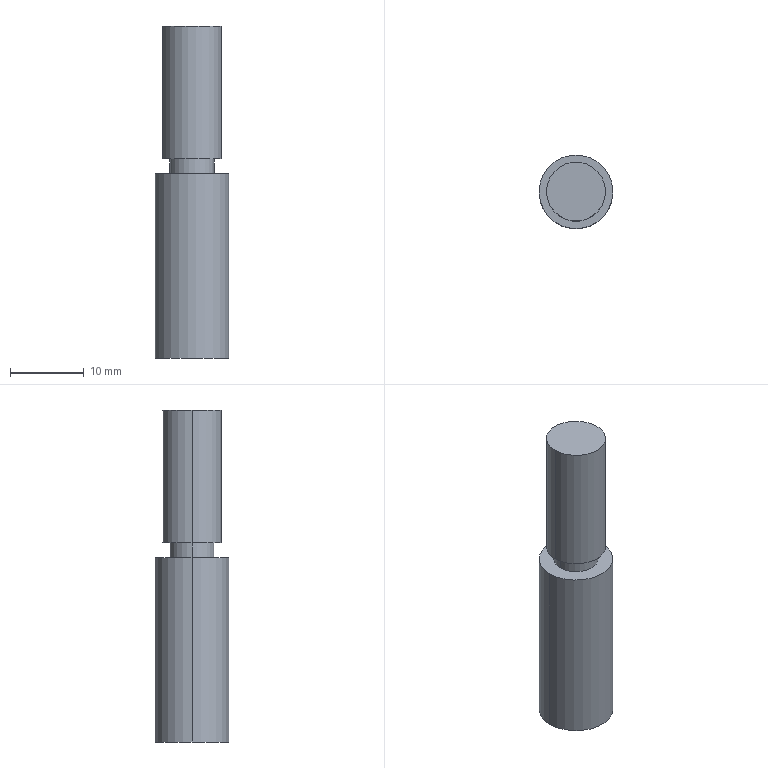Part | SolidWorks | features ICE 2, Extrusion 1 | 1 solid | 10 faces | box 10 x 10 x 45 mm | volume 2925 mm3 | cylinder 6 | plane 4 | commonest cylinder face diameters 6 x2 8 x2 10 x2
STEP:
#1=CARTESIAN_POINT('',(4.,0.,45.));
#2=VERTEX_POINT('',#1);
#3=CARTESIAN_POINT('',(-4.,0.,45.));
#4=VERTEX_POINT('',#3);
#5=CARTESIAN_POINT('',(0.,0.,45.));
#6=DIRECTION('',(0.,0.,1.));
#7=DIRECTION('',(1.,0.,0.));
#8=AXIS2_PLACEMENT_3D('',#5,#6,#7);
#9=CIRCLE('',#8,4.);
#10=EDGE_CURVE('',#2,#4,#9,.T.);
#11=ORIENTED_EDGE('',*,*,#10,.F.);
#12=CARTESIAN_POINT('',(4.,0.,27.));
#13=VERTEX_POINT('',#12);
#14=CARTESIAN_POINT('',(4.,0.,45.));
#15=DIRECTION('',(0.,0.,-1.));
#16=VECTOR('',#15,1000.);
#17=LINE('',#14,#16);
#18=EDGE_CURVE('',#2,#13,#17,.T.);
#19=ORIENTED_EDGE('',*,*,#18,.T.);
#20=CARTESIAN_POINT('',(-4.,0.,27.));
#21=VERTEX_POINT('',#20);
#22=CARTESIAN_POINT('',(0.,0.,27.));
#23=DIRECTION('',(0.,0.,1.));
#24=DIRECTION('',(1.,0.,0.));
#25=AXIS2_PLACEMENT_3D('',#22,#23,#24);
#26=CIRCLE('',#25,4.);
#27=EDGE_CURVE('',#13,#21,#26,.T.);
#28=ORIENTED_EDGE('',*,*,#27,.T.);
#29=CARTESIAN_POINT('',(-4.,0.,45.));
#30=DIRECTION('',(0.,0.,-1.));
#31=VECTOR('',#30,1000.);
#32=LINE('',#29,#31);
#33=EDGE_CURVE('',#4,#21,#32,.T.);
#34=ORIENTED_EDGE('',*,*,#33,.F.);
#35=EDGE_LOOP('',(#11,#19,#28,#34));
#36=FACE_OUTER_BOUND('',#35,.T.);
#37=CARTESIAN_POINT('',(0.,0.,45.));
#38=DIRECTION('',(0.,0.,-1.));
#39=DIRECTION('',(-1.,0.,0.));
#40=AXIS2_PLACEMENT_3D('',#37,#38,#39);
#41=CYLINDRICAL_SURFACE('',#40,4.);
#42=ADVANCED_FACE('',(#36),#41,.T.);
#43=CARTESIAN_POINT('',(3.,0.,27.));
#44=VERTEX_POINT('',#43);
#45=CARTESIAN_POINT('',(-3.,0.,27.));
#46=VERTEX_POINT('',#45);
#47=CARTESIAN_POINT('',(0.,0.,27.));
#48=DIRECTION('',(0.,0.,1.));
#49=DIRECTION('',(1.,0.,0.));
#50=AXIS2_PLACEMENT_3D('',#47,#48,#49);
#51=CIRCLE('',#50,3.);
#52=EDGE_CURVE('',#44,#46,#51,.T.);
#53=ORIENTED_EDGE('',*,*,#52,.F.);
#54=CARTESIAN_POINT('',(3.,0.,25.));
#55=VERTEX_POINT('',#54);
#56=CARTESIAN_POINT('',(3.,0.,27.));
#57=DIRECTION('',(0.,0.,-1.));
#58=VECTOR('',#57,1000.);
#59=LINE('',#56,#58);
#60=EDGE_CURVE('',#44,#55,#59,.T.);
#61=ORIENTED_EDGE('',*,*,#60,.T.);
#62=CARTESIAN_POINT('',(-3.,0.,25.));
#63=VERTEX_POINT('',#62);
#64=CARTESIAN_POINT('',(0.,0.,25.));
#65=DIRECTION('',(0.,0.,1.));
#66=DIRECTION('',(1.,0.,0.));
#67=AXIS2_PLACEMENT_3D('',#64,#65,#66);
#68=CIRCLE('',#67,3.);
#69=EDGE_CURVE('',#55,#63,#68,.T.);
#70=ORIENTED_EDGE('',*,*,#69,.T.);
#71=CARTESIAN_POINT('',(-3.,0.,27.));
#72=DIRECTION('',(0.,0.,-1.));
#73=VECTOR('',#72,1000.);
#74=LINE('',#71,#73);
#75=EDGE_CURVE('',#46,#63,#74,.T.);
#76=ORIENTED_EDGE('',*,*,#75,.F.);
#77=EDGE_LOOP('',(#53,#61,#70,#76));
#78=FACE_OUTER_BOUND('',#77,.T.);
#79=CARTESIAN_POINT('',(0.,0.,27.));
#80=DIRECTION('',(0.,0.,-1.));
#81=DIRECTION('',(-1.,0.,0.));
#82=AXIS2_PLACEMENT_3D('',#79,#80,#81);
#83=CYLINDRICAL_SURFACE('',#82,3.);
#84=ADVANCED_FACE('',(#78),#83,.T.);
#85=CARTESIAN_POINT('',(5.,0.,25.));
#86=VERTEX_POINT('',#85);
#87=CARTESIAN_POINT('',(-5.,0.,25.));
#88=VERTEX_POINT('',#87);
#89=CARTESIAN_POINT('',(0.,0.,25.));
#90=DIRECTION('',(0.,0.,1.));
#91=DIRECTION('',(1.,0.,0.));
#92=AXIS2_PLACEMENT_3D('',#89,#90,#91);
#93=CIRCLE('',#92,5.);
#94=EDGE_CURVE('',#86,#88,#93,.T.);
#95=ORIENTED_EDGE('',*,*,#94,.F.);
#96=CARTESIAN_POINT('',(5.,0.,0.));
#97=VERTEX_POINT('',#96);
#98=CARTESIAN_POINT('',(5.,0.,25.));
#99=DIRECTION('',(0.,0.,-1.));
#100=VECTOR('',#99,1000.);
#101=LINE('',#98,#100);
#102=EDGE_CURVE('',#86,#97,#101,.T.);
#103=ORIENTED_EDGE('',*,*,#102,.T.);
#104=CARTESIAN_POINT('',(-5.,0.,0.));
#105=VERTEX_POINT('',#104);
#106=CARTESIAN_POINT('',(0.,0.,0.));
#107=DIRECTION('',(0.,0.,1.));
#108=DIRECTION('',(1.,0.,0.));
#109=AXIS2_PLACEMENT_3D('',#106,#107,#108);
#110=CIRCLE('',#109,5.);
#111=EDGE_CURVE('',#97,#105,#110,.T.);
#112=ORIENTED_EDGE('',*,*,#111,.T.);
#113=CARTESIAN_POINT('',(-5.,0.,25.));
#114=DIRECTION('',(0.,0.,-1.));
#115=VECTOR('',#114,1000.);
#116=LINE('',#113,#115);
#117=EDGE_CURVE('',#88,#105,#116,.T.);
#118=ORIENTED_EDGE('',*,*,#117,.F.);
#119=EDGE_LOOP('',(#95,#103,#112,#118));
#120=FACE_OUTER_BOUND('',#119,.T.);
#121=CARTESIAN_POINT('',(0.,0.,25.));
#122=DIRECTION('',(0.,0.,-1.));
#123=DIRECTION('',(-1.,0.,0.));
#124=AXIS2_PLACEMENT_3D('',#121,#122,#123);
#125=CYLINDRICAL_SURFACE('',#124,5.);
#126=ADVANCED_FACE('',(#120),#125,.T.);
#127=ORIENTED_EDGE('',*,*,#102,.F.);
#128=CARTESIAN_POINT('',(0.,0.,25.));
#129=DIRECTION('',(0.,0.,1.));
#130=DIRECTION('',(1.,0.,0.));
#131=AXIS2_PLACEMENT_3D('',#128,#129,#130);
#132=CIRCLE('',#131,5.);
#133=EDGE_CURVE('',#88,#86,#132,.T.);
#134=ORIENTED_EDGE('',*,*,#133,.F.);
#135=ORIENTED_EDGE('',*,*,#117,.T.);
#136=CARTESIAN_POINT('',(0.,0.,0.));
#137=DIRECTION('',(0.,0.,1.));
#138=DIRECTION('',(1.,0.,0.));
#139=AXIS2_PLACEMENT_3D('',#136,#137,#138);
#140=CIRCLE('',#139,5.);
#141=EDGE_CURVE('',#105,#97,#140,.T.);
#142=ORIENTED_EDGE('',*,*,#141,.T.);
#143=EDGE_LOOP('',(#127,#134,#135,#142));
#144=FACE_OUTER_BOUND('',#143,.T.);
#145=CARTESIAN_POINT('',(0.,0.,25.));
#146=DIRECTION('',(0.,0.,-1.));
#147=DIRECTION('',(-1.,0.,0.));
#148=AXIS2_PLACEMENT_3D('',#145,#146,#147);
#149=CYLINDRICAL_SURFACE('',#148,5.);
#150=ADVANCED_FACE('',(#144),#149,.T.);
#151=ORIENTED_EDGE('',*,*,#133,.T.);
#152=ORIENTED_EDGE('',*,*,#94,.T.);
#153=EDGE_LOOP('',(#151,#152));
#154=FACE_OUTER_BOUND('',#153,.T.);
#155=CARTESIAN_POINT('',(0.,0.,25.));
#156=DIRECTION('',(0.,0.,1.));
#157=DIRECTION('',(1.,0.,0.));
#158=AXIS2_PLACEMENT_3D('',#155,#156,#157);
#159=CIRCLE('',#158,3.);
#160=EDGE_CURVE('',#63,#55,#159,.T.);
#161=ORIENTED_EDGE('',*,*,#160,.F.);
#162=ORIENTED_EDGE('',*,*,#69,.F.);
#163=EDGE_LOOP('',(#161,#162));
#164=FACE_BOUND('',#163,.T.);
#165=CARTESIAN_POINT('',(0.,0.,25.));
#166=DIRECTION('',(0.,0.,1.));
#167=DIRECTION('',(1.,0.,0.));
#168=AXIS2_PLACEMENT_3D('',#165,#166,#167);
#169=PLANE('',#168);
#170=ADVANCED_FACE('',(#154,#164),#169,.T.);
#171=ORIENTED_EDGE('',*,*,#141,.F.);
#172=ORIENTED_EDGE('',*,*,#111,.F.);
#173=EDGE_LOOP('',(#171,#172));
#174=FACE_OUTER_BOUND('',#173,.T.);
#175=CARTESIAN_POINT('',(0.,0.,0.));
#176=DIRECTION('',(0.,0.,1.));
#177=DIRECTION('',(1.,0.,0.));
#178=AXIS2_PLACEMENT_3D('',#175,#176,#177);
#179=PLANE('',#178);
#180=ADVANCED_FACE('',(#174),#179,.F.);
#181=CARTESIAN_POINT('',(0.,0.,27.));
#182=DIRECTION('',(0.,0.,1.));
#183=DIRECTION('',(1.,0.,0.));
#184=AXIS2_PLACEMENT_3D('',#181,#182,#183);
#185=CIRCLE('',#184,3.);
#186=EDGE_CURVE('',#46,#44,#185,.T.);
#187=ORIENTED_EDGE('',*,*,#186,.T.);
#188=ORIENTED_EDGE('',*,*,#52,.T.);
#189=EDGE_LOOP('',(#187,#188));
#190=FACE_BOUND('',#189,.T.);
#191=CARTESIAN_POINT('',(0.,0.,27.));
#192=DIRECTION('',(0.,0.,1.));
#193=DIRECTION('',(1.,0.,0.));
#194=AXIS2_PLACEMENT_3D('',#191,#192,#193);
#195=CIRCLE('',#194,4.);
#196=EDGE_CURVE('',#21,#13,#195,.T.);
#197=ORIENTED_EDGE('',*,*,#196,.F.);
#198=ORIENTED_EDGE('',*,*,#27,.F.);
#199=EDGE_LOOP('',(#197,#198));
#200=FACE_OUTER_BOUND('',#199,.T.);
#201=CARTESIAN_POINT('',(0.,0.,27.));
#202=DIRECTION('',(0.,0.,1.));
#203=DIRECTION('',(1.,0.,0.));
#204=AXIS2_PLACEMENT_3D('',#201,#202,#203);
#205=PLANE('',#204);
#206=ADVANCED_FACE('',(#190,#200),#205,.F.);
#207=ORIENTED_EDGE('',*,*,#60,.F.);
#208=ORIENTED_EDGE('',*,*,#186,.F.);
#209=ORIENTED_EDGE('',*,*,#75,.T.);
#210=ORIENTED_EDGE('',*,*,#160,.T.);
#211=EDGE_LOOP('',(#207,#208,#209,#210));
#212=FACE_OUTER_BOUND('',#211,.T.);
#213=CARTESIAN_POINT('',(0.,0.,27.));
#214=DIRECTION('',(0.,0.,-1.));
#215=DIRECTION('',(-1.,0.,0.));
#216=AXIS2_PLACEMENT_3D('',#213,#214,#215);
#217=CYLINDRICAL_SURFACE('',#216,3.);
#218=ADVANCED_FACE('',(#212),#217,.T.);
#219=CARTESIAN_POINT('',(0.,0.,45.));
#220=DIRECTION('',(0.,0.,1.));
#221=DIRECTION('',(1.,0.,0.));
#222=AXIS2_PLACEMENT_3D('',#219,#220,#221);
#223=CIRCLE('',#222,4.);
#224=EDGE_CURVE('',#4,#2,#223,.T.);
#225=ORIENTED_EDGE('',*,*,#224,.T.);
#226=ORIENTED_EDGE('',*,*,#10,.T.);
#227=EDGE_LOOP('',(#225,#226));
#228=FACE_OUTER_BOUND('',#227,.T.);
#229=CARTESIAN_POINT('',(0.,0.,45.));
#230=DIRECTION('',(0.,0.,1.));
#231=DIRECTION('',(1.,0.,0.));
#232=AXIS2_PLACEMENT_3D('',#229,#230,#231);
#233=PLANE('',#232);
#234=ADVANCED_FACE('',(#228),#233,.T.);
#235=ORIENTED_EDGE('',*,*,#18,.F.);
#236=ORIENTED_EDGE('',*,*,#224,.F.);
#237=ORIENTED_EDGE('',*,*,#33,.T.);
#238=ORIENTED_EDGE('',*,*,#196,.T.);
#239=EDGE_LOOP('',(#235,#236,#237,#238));
#240=FACE_OUTER_BOUND('',#239,.T.);
#241=CARTESIAN_POINT('',(0.,0.,45.));
#242=DIRECTION('',(0.,0.,-1.));
#243=DIRECTION('',(-1.,0.,0.));
#244=AXIS2_PLACEMENT_3D('',#241,#242,#243);
#245=CYLINDRICAL_SURFACE('',#244,4.);
#246=ADVANCED_FACE('',(#240),#245,.T.);
#247=CLOSED_SHELL('',(#42,#84,#126,#150,#170,#180,#206,#218,#234,#246));
#248=MANIFOLD_SOLID_BREP('',#247);
#249=CARTESIAN_POINT('',(0.,0.,0.));
#250=DIRECTION('',(0.,0.,1.));
#251=DIRECTION('',(1.,0.,0.));
#252=AXIS2_PLACEMENT_3D('',#249,#250,#251);
#253=(LENGTH_UNIT()NAMED_UNIT(*)SI_UNIT(.MILLI.,.METRE.));
#254=UNCERTAINTY_MEASURE_WITH_UNIT(LENGTH_MEASURE(0.00001),#253,'','');
#255=(NAMED_UNIT(*)PLANE_ANGLE_UNIT()SI_UNIT($,.RADIAN.));
#256=(NAMED_UNIT(*)SI_UNIT($,.STERADIAN.)SOLID_ANGLE_UNIT());
#257=(GEOMETRIC_REPRESENTATION_CONTEXT(3)GLOBAL_UNCERTAINTY_ASSIGNED_CONTEXT((#254))GLOBAL_UNIT_ASSIGNED_CONTEXT((#253,#255,#256))REPRESENTATION_CONTEXT('',''));
#258=ADVANCED_BREP_SHAPE_REPRESENTATION('',(#248,#252),#257);